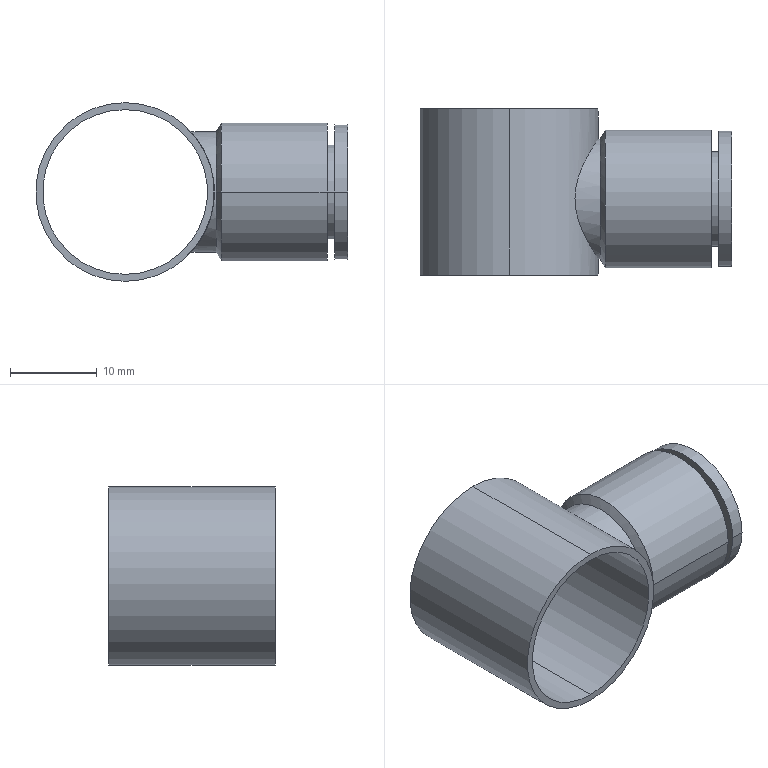Part | SolidWorks | features RefAxis 3, BaseBody 1 | 1 solid | 22 faces | box 36 x 19.2 x 20.6 mm | volume 2754 mm3 | cylinder 14 | plane 6 | cone 2 | commonest cylinder face diameters 10 x2 10.95 x2 13.9 x2 15.6 x2 15.9 x2 19 x2
STEP:
#1=CARTESIAN_POINT('',(0.,0.,-9.5));
#2=VERTEX_POINT('',#1);
#3=CARTESIAN_POINT('',(0.,0.,9.5));
#4=VERTEX_POINT('',#3);
#5=CARTESIAN_POINT('',(0.,0.,0.));
#6=DIRECTION('',(0.,1.,0.));
#7=DIRECTION('',(0.,0.,1.));
#8=AXIS2_PLACEMENT_3D('',#5,#6,#7);
#9=CIRCLE('',#8,9.5);
#10=EDGE_CURVE('',#2,#4,#9,.T.);
#11=ORIENTED_EDGE('',*,*,#10,.F.);
#12=CARTESIAN_POINT('',(0.,19.2,-9.5));
#13=VERTEX_POINT('',#12);
#14=CARTESIAN_POINT('',(0.,0.,-9.5));
#15=DIRECTION('',(0.,1.,0.));
#16=VECTOR('',#15,1000.);
#17=LINE('',#14,#16);
#18=EDGE_CURVE('',#2,#13,#17,.T.);
#19=ORIENTED_EDGE('',*,*,#18,.T.);
#20=CARTESIAN_POINT('',(0.,19.2,9.5));
#21=VERTEX_POINT('',#20);
#22=CARTESIAN_POINT('',(0.,19.2,0.));
#23=DIRECTION('',(0.,-1.,0.));
#24=DIRECTION('',(0.,0.,1.));
#25=AXIS2_PLACEMENT_3D('',#22,#23,#24);
#26=CIRCLE('',#25,9.5);
#27=EDGE_CURVE('',#21,#13,#26,.T.);
#28=ORIENTED_EDGE('',*,*,#27,.F.);
#29=CARTESIAN_POINT('',(0.,0.,9.5));
#30=DIRECTION('',(0.,1.,0.));
#31=VECTOR('',#30,1000.);
#32=LINE('',#29,#31);
#33=EDGE_CURVE('',#4,#21,#32,.T.);
#34=ORIENTED_EDGE('',*,*,#33,.F.);
#35=EDGE_LOOP('',(#11,#19,#28,#34));
#36=FACE_OUTER_BOUND('',#35,.T.);
#37=CARTESIAN_POINT('',(0.,0.,0.));
#38=DIRECTION('',(0.,1.,0.));
#39=DIRECTION('',(0.,0.,1.));
#40=AXIS2_PLACEMENT_3D('',#37,#38,#39);
#41=CYLINDRICAL_SURFACE('',#40,9.5);
#42=ADVANCED_FACE('',(#36),#41,.F.);
#43=CARTESIAN_POINT('',(10.3,1.85,0.));
#44=VERTEX_POINT('',#43);
#45=CARTESIAN_POINT('',(10.3,15.75,0.));
#46=VERTEX_POINT('',#45);
#47=CARTESIAN_POINT('',(10.3,1.85,0.));
#48=CARTESIAN_POINT('',(10.3,1.85,0.2364));
#49=CARTESIAN_POINT('',(10.292,1.862,0.4747));
#50=CARTESIAN_POINT('',(10.26,1.91,0.9419));
#51=CARTESIAN_POINT('',(10.236,1.946,1.173));
#52=CARTESIAN_POINT('',(10.142,2.086,1.856));
#53=CARTESIAN_POINT('',(10.048,2.227,2.305));
#54=CARTESIAN_POINT('',(9.818,2.585,3.145));
#55=CARTESIAN_POINT('',(9.681,2.802,3.54));
#56=CARTESIAN_POINT('',(9.376,3.308,4.283));
#57=CARTESIAN_POINT('',(9.212,3.591,4.621));
#58=CARTESIAN_POINT('',(8.874,4.213,5.24));
#59=CARTESIAN_POINT('',(8.7,4.557,5.522));
#60=CARTESIAN_POINT('',(8.368,5.287,6.013));
#61=CARTESIAN_POINT('',(8.21,5.674,6.223));
#62=CARTESIAN_POINT('',(7.933,6.5,6.574));
#63=CARTESIAN_POINT('',(7.812,6.944,6.713));
#64=CARTESIAN_POINT('',(7.689,7.624,6.854));
#65=CARTESIAN_POINT('',(7.657,7.854,6.889));
#66=CARTESIAN_POINT('',(7.613,8.322,6.938));
#67=CARTESIAN_POINT('',(7.602,8.561,6.95));
#68=CARTESIAN_POINT('',(7.602,9.269,6.95));
#69=CARTESIAN_POINT('',(7.646,9.734,6.903));
#70=CARTESIAN_POINT('',(7.811,10.651,6.715));
#71=CARTESIAN_POINT('',(7.929,11.089,6.578));
#72=CARTESIAN_POINT('',(8.138,11.713,6.314));
#73=CARTESIAN_POINT('',(8.214,11.917,6.216));
#74=CARTESIAN_POINT('',(8.371,12.309,6.003));
#75=CARTESIAN_POINT('',(8.452,12.498,5.889));
#76=CARTESIAN_POINT('',(8.7,13.044,5.521));
#77=CARTESIAN_POINT('',(8.872,13.382,5.244));
#78=CARTESIAN_POINT('',(9.127,13.852,4.777));
#79=CARTESIAN_POINT('',(9.211,14.003,4.613));
#80=CARTESIAN_POINT('',(9.374,14.285,4.273));
#81=CARTESIAN_POINT('',(9.452,14.418,4.097));
#82=CARTESIAN_POINT('',(9.678,14.793,3.548));
#83=CARTESIAN_POINT('',(9.815,15.01,3.155));
#84=CARTESIAN_POINT('',(10.048,15.372,2.307));
#85=CARTESIAN_POINT('',(10.14,15.511,1.865));
#86=CARTESIAN_POINT('',(10.266,15.7,0.9518));
#87=CARTESIAN_POINT('',(10.3,15.75,0.4749));
#88=CARTESIAN_POINT('',(10.3,15.75,0.));
#89=B_SPLINE_CURVE_WITH_KNOTS('',3,(#47,#48,#49,#50,#51,#52,#53,#54,#55,#56,#57,#58,#59,#60,#61,#62,#63,#64,#65,#66,#67,#68,#69,#70,#71,#72,#73,#74,#75,#76,#77,#78,#79,#80,#81,#82,#83,#84,#85,#86,#87,#88),.UNSPECIFIED.,.F.,.F.,(4,2,2,2,2,2,2,2,2,2,2,2,2,2,2,2,2,2,2,2,4),(0.02215,0.02285,0.02355,0.02495,0.02635,0.02775,0.02915,0.03055,0.03196,0.03266,0.03336,0.03476,0.03616,0.03686,0.03756,0.03896,0.03966,0.04036,0.04176,0.04317,0.04457),.UNSPECIFIED.);
#90=EDGE_CURVE('',#44,#46,#89,.T.);
#91=ORIENTED_EDGE('',*,*,#90,.T.);
#92=CARTESIAN_POINT('',(10.3,15.75,0.));
#93=CARTESIAN_POINT('',(10.3,15.75,-0.2383));
#94=CARTESIAN_POINT('',(10.292,15.738,-0.4775));
#95=CARTESIAN_POINT('',(10.259,15.689,-0.9459));
#96=CARTESIAN_POINT('',(10.235,15.654,-1.177));
#97=CARTESIAN_POINT('',(10.173,15.56,-1.632));
#98=CARTESIAN_POINT('',(10.134,15.502,-1.856));
#99=CARTESIAN_POINT('',(10.043,15.363,-2.298));
#100=CARTESIAN_POINT('',(9.99,15.283,-2.516));
#101=CARTESIAN_POINT('',(9.817,15.013,-3.148));
#102=CARTESIAN_POINT('',(9.68,14.796,-3.542));
#103=CARTESIAN_POINT('',(9.452,14.418,-4.097));
#104=CARTESIAN_POINT('',(9.372,14.283,-4.276));
#105=CARTESIAN_POINT('',(9.209,13.999,-4.617));
#106=CARTESIAN_POINT('',(9.126,13.851,-4.779));
#107=CARTESIAN_POINT('',(8.873,13.383,-5.243));
#108=CARTESIAN_POINT('',(8.7,13.043,-5.522));
#109=CARTESIAN_POINT('',(8.365,12.307,-6.017));
#110=CARTESIAN_POINT('',(8.208,11.919,-6.227));
#111=CARTESIAN_POINT('',(8.001,11.302,-6.488));
#112=CARTESIAN_POINT('',(7.937,11.091,-6.566));
#113=CARTESIAN_POINT('',(7.822,10.654,-6.702));
#114=CARTESIAN_POINT('',(7.771,10.428,-6.761));
#115=CARTESIAN_POINT('',(7.647,9.742,-6.902));
#116=CARTESIAN_POINT('',(7.602,9.277,-6.95));
#117=CARTESIAN_POINT('',(7.602,8.562,-6.95));
#118=CARTESIAN_POINT('',(7.613,8.325,-6.938));
#119=CARTESIAN_POINT('',(7.656,7.858,-6.89));
#120=CARTESIAN_POINT('',(7.688,7.627,-6.854));
#121=CARTESIAN_POINT('',(7.771,7.172,-6.761));
#122=CARTESIAN_POINT('',(7.822,6.945,-6.702));
#123=CARTESIAN_POINT('',(7.937,6.507,-6.565));
#124=CARTESIAN_POINT('',(8.002,6.294,-6.486));
#125=CARTESIAN_POINT('',(8.21,5.674,-6.224));
#126=CARTESIAN_POINT('',(8.37,5.283,-6.011));
#127=CARTESIAN_POINT('',(8.705,4.546,-5.514));
#128=CARTESIAN_POINT('',(8.877,4.208,-5.235));
#129=CARTESIAN_POINT('',(9.215,3.585,-4.615));
#130=CARTESIAN_POINT('',(9.382,3.298,-4.269));
#131=CARTESIAN_POINT('',(9.684,2.798,-3.532));
#132=CARTESIAN_POINT('',(9.82,2.583,-3.139));
#133=CARTESIAN_POINT('',(10.049,2.226,-2.301));
#134=CARTESIAN_POINT('',(10.143,2.085,-1.85));
#135=CARTESIAN_POINT('',(10.267,1.898,-0.939));
#136=CARTESIAN_POINT('',(10.3,1.85,-0.4743));
#137=CARTESIAN_POINT('',(10.3,1.85,0.));
#138=B_SPLINE_CURVE_WITH_KNOTS('',3,(#92,#93,#94,#95,#96,#97,#98,#99,#100,#101,#102,#103,#104,#105,#106,#107,#108,#109,#110,#111,#112,#113,#114,#115,#116,#117,#118,#119,#120,#121,#122,#123,#124,#125,#126,#127,#128,#129,#130,#131,#132,#133,#134,#135,#136,#137),.UNSPECIFIED.,.F.,.F.,(4,2,2,2,2,2,2,2,2,2,2,2,2,2,2,2,2,2,2,2,2,2,4),(0.04457,0.04527,0.04597,0.04668,0.04738,0.04878,0.04949,0.05019,0.0516,0.053,0.05371,0.05441,0.05581,0.05652,0.05722,0.05792,0.05863,0.06003,0.06144,0.06284,0.06425,0.06566,0.06706),.UNSPECIFIED.);
#139=EDGE_CURVE('',#46,#44,#138,.T.);
#140=ORIENTED_EDGE('',*,*,#139,.T.);
#141=EDGE_LOOP('',(#91,#140));
#142=FACE_BOUND('',#141,.T.);
#143=CARTESIAN_POINT('',(0.,19.2,-10.3));
#144=VERTEX_POINT('',#143);
#145=CARTESIAN_POINT('',(0.,19.2,10.3));
#146=VERTEX_POINT('',#145);
#147=CARTESIAN_POINT('',(0.,19.2,0.));
#148=DIRECTION('',(0.,-1.,0.));
#149=DIRECTION('',(0.,0.,-1.));
#150=AXIS2_PLACEMENT_3D('',#147,#148,#149);
#151=CIRCLE('',#150,10.3);
#152=EDGE_CURVE('',#144,#146,#151,.T.);
#153=ORIENTED_EDGE('',*,*,#152,.T.);
#154=CARTESIAN_POINT('',(0.,0.,10.3));
#155=VERTEX_POINT('',#154);
#156=CARTESIAN_POINT('',(0.,19.2,10.3));
#157=DIRECTION('',(0.,-1.,0.));
#158=VECTOR('',#157,1000.);
#159=LINE('',#156,#158);
#160=EDGE_CURVE('',#146,#155,#159,.T.);
#161=ORIENTED_EDGE('',*,*,#160,.T.);
#162=CARTESIAN_POINT('',(0.,0.,-10.3));
#163=VERTEX_POINT('',#162);
#164=CARTESIAN_POINT('',(0.,0.,0.));
#165=DIRECTION('',(0.,1.,0.));
#166=DIRECTION('',(0.,0.,-1.));
#167=AXIS2_PLACEMENT_3D('',#164,#165,#166);
#168=CIRCLE('',#167,10.3);
#169=EDGE_CURVE('',#155,#163,#168,.T.);
#170=ORIENTED_EDGE('',*,*,#169,.T.);
#171=CARTESIAN_POINT('',(0.,19.2,-10.3));
#172=DIRECTION('',(0.,-1.,0.));
#173=VECTOR('',#172,1000.);
#174=LINE('',#171,#173);
#175=EDGE_CURVE('',#144,#163,#174,.T.);
#176=ORIENTED_EDGE('',*,*,#175,.F.);
#177=EDGE_LOOP('',(#153,#161,#170,#176));
#178=FACE_OUTER_BOUND('',#177,.T.);
#179=CARTESIAN_POINT('',(0.,19.2,0.));
#180=DIRECTION('',(0.,-1.,0.));
#181=DIRECTION('',(0.,0.,-1.));
#182=AXIS2_PLACEMENT_3D('',#179,#180,#181);
#183=CYLINDRICAL_SURFACE('',#182,10.3);
#184=ADVANCED_FACE('',(#142,#178),#183,.T.);
#185=CARTESIAN_POINT('',(10.523,1.85,0.));
#186=VERTEX_POINT('',#185);
#187=CARTESIAN_POINT('',(10.523,15.75,0.));
#188=VERTEX_POINT('',#187);
#189=CARTESIAN_POINT('',(10.523,8.8,0.));
#190=DIRECTION('',(-1.,0.,0.));
#191=DIRECTION('',(0.,-1.,0.));
#192=AXIS2_PLACEMENT_3D('',#189,#190,#191);
#193=CIRCLE('',#192,6.95);
#194=EDGE_CURVE('',#186,#188,#193,.T.);
#195=ORIENTED_EDGE('',*,*,#194,.T.);
#196=CARTESIAN_POINT('',(25.7,15.75,0.));
#197=DIRECTION('',(-1.,0.,0.));
#198=VECTOR('',#197,1000.);
#199=LINE('',#196,#198);
#200=EDGE_CURVE('',#188,#46,#199,.T.);
#201=ORIENTED_EDGE('',*,*,#200,.T.);
#202=ORIENTED_EDGE('',*,*,#90,.F.);
#203=CARTESIAN_POINT('',(25.7,1.85,0.));
#204=DIRECTION('',(-1.,0.,0.));
#205=VECTOR('',#204,1000.);
#206=LINE('',#203,#205);
#207=EDGE_CURVE('',#186,#44,#206,.T.);
#208=ORIENTED_EDGE('',*,*,#207,.F.);
#209=EDGE_LOOP('',(#195,#201,#202,#208));
#210=FACE_OUTER_BOUND('',#209,.T.);
#211=CARTESIAN_POINT('',(25.7,8.8,0.));
#212=DIRECTION('',(-1.,0.,0.));
#213=DIRECTION('',(0.,-1.,0.));
#214=AXIS2_PLACEMENT_3D('',#211,#212,#213);
#215=CYLINDRICAL_SURFACE('',#214,6.95);
#216=ADVANCED_FACE('',(#210),#215,.T.);
#217=ORIENTED_EDGE('',*,*,#194,.F.);
#218=CARTESIAN_POINT('',(11.1,0.85,0.));
#219=VERTEX_POINT('',#218);
#220=CARTESIAN_POINT('',(11.1,0.85,0.));
#221=DIRECTION('',(0.5,-0.866,0.));
#222=VECTOR('',#221,1000.);
#223=LINE('',#220,#222);
#224=EDGE_CURVE('',#186,#219,#223,.T.);
#225=ORIENTED_EDGE('',*,*,#224,.T.);
#226=CARTESIAN_POINT('',(11.1,16.75,0.));
#227=VERTEX_POINT('',#226);
#228=CARTESIAN_POINT('',(11.1,8.8,0.));
#229=DIRECTION('',(-1.,0.,0.));
#230=DIRECTION('',(0.,1.,0.));
#231=AXIS2_PLACEMENT_3D('',#228,#229,#230);
#232=CIRCLE('',#231,7.95);
#233=EDGE_CURVE('',#219,#227,#232,.T.);
#234=ORIENTED_EDGE('',*,*,#233,.T.);
#235=CARTESIAN_POINT('',(11.1,16.75,0.));
#236=DIRECTION('',(0.5,0.866,0.));
#237=VECTOR('',#236,1000.);
#238=LINE('',#235,#237);
#239=EDGE_CURVE('',#188,#227,#238,.T.);
#240=ORIENTED_EDGE('',*,*,#239,.F.);
#241=EDGE_LOOP('',(#217,#225,#234,#240));
#242=FACE_OUTER_BOUND('',#241,.T.);
#243=CARTESIAN_POINT('',(11.1,8.8,0.));
#244=DIRECTION('',(1.,0.,0.));
#245=DIRECTION('',(0.,1.,0.));
#246=AXIS2_PLACEMENT_3D('',#243,#244,#245);
#247=CONICAL_SURFACE('',#246,7.95,1.047);
#248=ADVANCED_FACE('',(#242),#247,.T.);
#249=CARTESIAN_POINT('',(23.3,0.85,0.));
#250=VERTEX_POINT('',#249);
#251=CARTESIAN_POINT('',(23.3,16.75,0.));
#252=VERTEX_POINT('',#251);
#253=CARTESIAN_POINT('',(23.3,8.8,0.));
#254=DIRECTION('',(-1.,0.,0.));
#255=DIRECTION('',(0.,-1.,0.));
#256=AXIS2_PLACEMENT_3D('',#253,#254,#255);
#257=CIRCLE('',#256,7.95);
#258=EDGE_CURVE('',#250,#252,#257,.T.);
#259=ORIENTED_EDGE('',*,*,#258,.T.);
#260=CARTESIAN_POINT('',(25.7,16.75,0.));
#261=DIRECTION('',(-1.,0.,0.));
#262=VECTOR('',#261,1000.);
#263=LINE('',#260,#262);
#264=EDGE_CURVE('',#252,#227,#263,.T.);
#265=ORIENTED_EDGE('',*,*,#264,.T.);
#266=ORIENTED_EDGE('',*,*,#233,.F.);
#267=CARTESIAN_POINT('',(25.7,0.85,0.));
#268=DIRECTION('',(-1.,0.,0.));
#269=VECTOR('',#268,1000.);
#270=LINE('',#267,#269);
#271=EDGE_CURVE('',#250,#219,#270,.T.);
#272=ORIENTED_EDGE('',*,*,#271,.F.);
#273=EDGE_LOOP('',(#259,#265,#266,#272));
#274=FACE_OUTER_BOUND('',#273,.T.);
#275=CARTESIAN_POINT('',(25.7,8.8,0.));
#276=DIRECTION('',(-1.,0.,0.));
#277=DIRECTION('',(0.,-1.,0.));
#278=AXIS2_PLACEMENT_3D('',#275,#276,#277);
#279=CYLINDRICAL_SURFACE('',#278,7.95);
#280=ADVANCED_FACE('',(#274),#279,.T.);
#281=CARTESIAN_POINT('',(24.2,3.325,0.));
#282=VERTEX_POINT('',#281);
#283=CARTESIAN_POINT('',(24.2,14.275,0.));
#284=VERTEX_POINT('',#283);
#285=CARTESIAN_POINT('',(24.2,8.8,0.));
#286=DIRECTION('',(-1.,0.,0.));
#287=DIRECTION('',(0.,-1.,0.));
#288=AXIS2_PLACEMENT_3D('',#285,#286,#287);
#289=CIRCLE('',#288,5.475);
#290=EDGE_CURVE('',#282,#284,#289,.T.);
#291=ORIENTED_EDGE('',*,*,#290,.T.);
#292=CARTESIAN_POINT('',(23.3,14.275,0.));
#293=VERTEX_POINT('',#292);
#294=CARTESIAN_POINT('',(25.7,14.275,0.));
#295=DIRECTION('',(-1.,0.,0.));
#296=VECTOR('',#295,1000.);
#297=LINE('',#294,#296);
#298=EDGE_CURVE('',#284,#293,#297,.T.);
#299=ORIENTED_EDGE('',*,*,#298,.T.);
#300=CARTESIAN_POINT('',(23.3,3.325,0.));
#301=VERTEX_POINT('',#300);
#302=CARTESIAN_POINT('',(23.3,8.8,0.));
#303=DIRECTION('',(1.,0.,0.));
#304=DIRECTION('',(0.,-1.,0.));
#305=AXIS2_PLACEMENT_3D('',#302,#303,#304);
#306=CIRCLE('',#305,5.475);
#307=EDGE_CURVE('',#293,#301,#306,.T.);
#308=ORIENTED_EDGE('',*,*,#307,.T.);
#309=CARTESIAN_POINT('',(25.7,3.325,0.));
#310=DIRECTION('',(-1.,0.,0.));
#311=VECTOR('',#310,1000.);
#312=LINE('',#309,#311);
#313=EDGE_CURVE('',#282,#301,#312,.T.);
#314=ORIENTED_EDGE('',*,*,#313,.F.);
#315=EDGE_LOOP('',(#291,#299,#308,#314));
#316=FACE_OUTER_BOUND('',#315,.T.);
#317=CARTESIAN_POINT('',(25.7,8.8,0.));
#318=DIRECTION('',(-1.,0.,0.));
#319=DIRECTION('',(0.,-1.,0.));
#320=AXIS2_PLACEMENT_3D('',#317,#318,#319);
#321=CYLINDRICAL_SURFACE('',#320,5.475);
#322=ADVANCED_FACE('',(#316),#321,.T.);
#323=CARTESIAN_POINT('',(25.7,1.,0.));
#324=VERTEX_POINT('',#323);
#325=CARTESIAN_POINT('',(25.7,16.6,0.));
#326=VERTEX_POINT('',#325);
#327=CARTESIAN_POINT('',(25.7,8.8,0.));
#328=DIRECTION('',(-1.,0.,0.));
#329=DIRECTION('',(0.,-1.,0.));
#330=AXIS2_PLACEMENT_3D('',#327,#328,#329);
#331=CIRCLE('',#330,7.8);
#332=EDGE_CURVE('',#324,#326,#331,.T.);
#333=ORIENTED_EDGE('',*,*,#332,.T.);
#334=CARTESIAN_POINT('',(24.2,16.6,0.));
#335=VERTEX_POINT('',#334);
#336=CARTESIAN_POINT('',(25.7,16.6,0.));
#337=DIRECTION('',(-1.,0.,0.));
#338=VECTOR('',#337,1000.);
#339=LINE('',#336,#338);
#340=EDGE_CURVE('',#326,#335,#339,.T.);
#341=ORIENTED_EDGE('',*,*,#340,.T.);
#342=CARTESIAN_POINT('',(24.2,1.,0.));
#343=VERTEX_POINT('',#342);
#344=CARTESIAN_POINT('',(24.2,8.8,0.));
#345=DIRECTION('',(1.,0.,0.));
#346=DIRECTION('',(0.,-1.,0.));
#347=AXIS2_PLACEMENT_3D('',#344,#345,#346);
#348=CIRCLE('',#347,7.8);
#349=EDGE_CURVE('',#335,#343,#348,.T.);
#350=ORIENTED_EDGE('',*,*,#349,.T.);
#351=CARTESIAN_POINT('',(25.7,1.,0.));
#352=DIRECTION('',(-1.,0.,0.));
#353=VECTOR('',#352,1000.);
#354=LINE('',#351,#353);
#355=EDGE_CURVE('',#324,#343,#354,.T.);
#356=ORIENTED_EDGE('',*,*,#355,.F.);
#357=EDGE_LOOP('',(#333,#341,#350,#356));
#358=FACE_OUTER_BOUND('',#357,.T.);
#359=CARTESIAN_POINT('',(25.7,8.8,0.));
#360=DIRECTION('',(-1.,0.,0.));
#361=DIRECTION('',(0.,-1.,0.));
#362=AXIS2_PLACEMENT_3D('',#359,#360,#361);
#363=CYLINDRICAL_SURFACE('',#362,7.8);
#364=ADVANCED_FACE('',(#358),#363,.T.);
#365=CARTESIAN_POINT('',(25.7,8.8,5.));
#366=VERTEX_POINT('',#365);
#367=CARTESIAN_POINT('',(25.7,8.8,-5.));
#368=VERTEX_POINT('',#367);
#369=CARTESIAN_POINT('',(25.7,8.8,0.));
#370=DIRECTION('',(1.,0.,0.));
#371=DIRECTION('',(0.,0.,1.));
#372=AXIS2_PLACEMENT_3D('',#369,#370,#371);
#373=CIRCLE('',#372,5.);
#374=EDGE_CURVE('',#366,#368,#373,.T.);
#375=ORIENTED_EDGE('',*,*,#374,.T.);
#376=CARTESIAN_POINT('',(10.1,8.8,-5.));
#377=VERTEX_POINT('',#376);
#378=CARTESIAN_POINT('',(10.1,8.8,-5.));
#379=DIRECTION('',(-1.,0.,0.));
#380=VECTOR('',#379,1000.);
#381=LINE('',#378,#380);
#382=EDGE_CURVE('',#368,#377,#381,.T.);
#383=ORIENTED_EDGE('',*,*,#382,.T.);
#384=CARTESIAN_POINT('',(10.1,8.8,5.));
#385=VERTEX_POINT('',#384);
#386=CARTESIAN_POINT('',(10.1,8.8,0.));
#387=DIRECTION('',(1.,0.,0.));
#388=DIRECTION('',(0.,0.,1.));
#389=AXIS2_PLACEMENT_3D('',#386,#387,#388);
#390=CIRCLE('',#389,5.);
#391=EDGE_CURVE('',#385,#377,#390,.T.);
#392=ORIENTED_EDGE('',*,*,#391,.F.);
#393=CARTESIAN_POINT('',(10.1,8.8,5.));
#394=DIRECTION('',(-1.,0.,0.));
#395=VECTOR('',#394,1000.);
#396=LINE('',#393,#395);
#397=EDGE_CURVE('',#366,#385,#396,.T.);
#398=ORIENTED_EDGE('',*,*,#397,.F.);
#399=EDGE_LOOP('',(#375,#383,#392,#398));
#400=FACE_OUTER_BOUND('',#399,.T.);
#401=CARTESIAN_POINT('',(10.1,8.8,0.));
#402=DIRECTION('',(-1.,0.,0.));
#403=DIRECTION('',(0.,0.,1.));
#404=AXIS2_PLACEMENT_3D('',#401,#402,#403);
#405=CYLINDRICAL_SURFACE('',#404,5.);
#406=ADVANCED_FACE('',(#400),#405,.F.);
#407=ORIENTED_EDGE('',*,*,#18,.F.);
#408=CARTESIAN_POINT('',(0.,0.,0.));
#409=DIRECTION('',(0.,1.,0.));
#410=DIRECTION('',(0.,0.,1.));
#411=AXIS2_PLACEMENT_3D('',#408,#409,#410);
#412=CIRCLE('',#411,9.5);
#413=EDGE_CURVE('',#4,#2,#412,.T.);
#414=ORIENTED_EDGE('',*,*,#413,.F.);
#415=ORIENTED_EDGE('',*,*,#33,.T.);
#416=CARTESIAN_POINT('',(0.,19.2,0.));
#417=DIRECTION('',(0.,-1.,0.));
#418=DIRECTION('',(0.,0.,1.));
#419=AXIS2_PLACEMENT_3D('',#416,#417,#418);
#420=CIRCLE('',#419,9.5);
#421=EDGE_CURVE('',#13,#21,#420,.T.);
#422=ORIENTED_EDGE('',*,*,#421,.F.);
#423=EDGE_LOOP('',(#407,#414,#415,#422));
#424=FACE_OUTER_BOUND('',#423,.T.);
#425=CARTESIAN_POINT('',(0.,0.,0.));
#426=DIRECTION('',(0.,1.,0.));
#427=DIRECTION('',(0.,0.,1.));
#428=AXIS2_PLACEMENT_3D('',#425,#426,#427);
#429=CYLINDRICAL_SURFACE('',#428,9.5);
#430=ADVANCED_FACE('',(#424),#429,.F.);
#431=ORIENTED_EDGE('',*,*,#152,.F.);
#432=CARTESIAN_POINT('',(0.,19.2,0.));
#433=DIRECTION('',(0.,-1.,0.));
#434=DIRECTION('',(0.,0.,-1.));
#435=AXIS2_PLACEMENT_3D('',#432,#433,#434);
#436=CIRCLE('',#435,10.3);
#437=EDGE_CURVE('',#146,#144,#436,.T.);
#438=ORIENTED_EDGE('',*,*,#437,.F.);
#439=EDGE_LOOP('',(#431,#438));
#440=FACE_OUTER_BOUND('',#439,.T.);
#441=ORIENTED_EDGE('',*,*,#27,.T.);
#442=ORIENTED_EDGE('',*,*,#421,.T.);
#443=EDGE_LOOP('',(#441,#442));
#444=FACE_BOUND('',#443,.T.);
#445=CARTESIAN_POINT('',(-10.3,19.2,0.));
#446=DIRECTION('',(0.,-1.,0.));
#447=DIRECTION('',(0.,0.,-1.));
#448=AXIS2_PLACEMENT_3D('',#445,#446,#447);
#449=PLANE('',#448);
#450=ADVANCED_FACE('',(#440,#444),#449,.F.);
#451=ORIENTED_EDGE('',*,*,#413,.T.);
#452=ORIENTED_EDGE('',*,*,#10,.T.);
#453=EDGE_LOOP('',(#451,#452));
#454=FACE_BOUND('',#453,.T.);
#455=CARTESIAN_POINT('',(0.,0.,0.));
#456=DIRECTION('',(0.,1.,0.));
#457=DIRECTION('',(0.,0.,-1.));
#458=AXIS2_PLACEMENT_3D('',#455,#456,#457);
#459=CIRCLE('',#458,10.3);
#460=EDGE_CURVE('',#163,#155,#459,.T.);
#461=ORIENTED_EDGE('',*,*,#460,.F.);
#462=ORIENTED_EDGE('',*,*,#169,.F.);
#463=EDGE_LOOP('',(#461,#462));
#464=FACE_OUTER_BOUND('',#463,.T.);
#465=CARTESIAN_POINT('',(0.,0.,0.));
#466=DIRECTION('',(0.,1.,0.));
#467=DIRECTION('',(0.,0.,1.));
#468=AXIS2_PLACEMENT_3D('',#465,#466,#467);
#469=PLANE('',#468);
#470=ADVANCED_FACE('',(#454,#464),#469,.F.);
#471=ORIENTED_EDGE('',*,*,#160,.F.);
#472=ORIENTED_EDGE('',*,*,#437,.T.);
#473=ORIENTED_EDGE('',*,*,#175,.T.);
#474=ORIENTED_EDGE('',*,*,#460,.T.);
#475=EDGE_LOOP('',(#471,#472,#473,#474));
#476=FACE_OUTER_BOUND('',#475,.T.);
#477=CARTESIAN_POINT('',(0.,19.2,0.));
#478=DIRECTION('',(0.,-1.,0.));
#479=DIRECTION('',(0.,0.,-1.));
#480=AXIS2_PLACEMENT_3D('',#477,#478,#479);
#481=CYLINDRICAL_SURFACE('',#480,10.3);
#482=ADVANCED_FACE('',(#476),#481,.T.);
#483=ORIENTED_EDGE('',*,*,#200,.F.);
#484=CARTESIAN_POINT('',(10.523,8.8,0.));
#485=DIRECTION('',(-1.,0.,0.));
#486=DIRECTION('',(0.,-1.,0.));
#487=AXIS2_PLACEMENT_3D('',#484,#485,#486);
#488=CIRCLE('',#487,6.95);
#489=EDGE_CURVE('',#188,#186,#488,.T.);
#490=ORIENTED_EDGE('',*,*,#489,.T.);
#491=ORIENTED_EDGE('',*,*,#207,.T.);
#492=ORIENTED_EDGE('',*,*,#139,.F.);
#493=EDGE_LOOP('',(#483,#490,#491,#492));
#494=FACE_OUTER_BOUND('',#493,.T.);
#495=CARTESIAN_POINT('',(25.7,8.8,0.));
#496=DIRECTION('',(-1.,0.,0.));
#497=DIRECTION('',(0.,-1.,0.));
#498=AXIS2_PLACEMENT_3D('',#495,#496,#497);
#499=CYLINDRICAL_SURFACE('',#498,6.95);
#500=ADVANCED_FACE('',(#494),#499,.T.);
#501=ORIENTED_EDGE('',*,*,#224,.F.);
#502=ORIENTED_EDGE('',*,*,#489,.F.);
#503=ORIENTED_EDGE('',*,*,#239,.T.);
#504=CARTESIAN_POINT('',(11.1,8.8,0.));
#505=DIRECTION('',(-1.,0.,0.));
#506=DIRECTION('',(0.,1.,0.));
#507=AXIS2_PLACEMENT_3D('',#504,#505,#506);
#508=CIRCLE('',#507,7.95);
#509=EDGE_CURVE('',#227,#219,#508,.T.);
#510=ORIENTED_EDGE('',*,*,#509,.T.);
#511=EDGE_LOOP('',(#501,#502,#503,#510));
#512=FACE_OUTER_BOUND('',#511,.T.);
#513=CARTESIAN_POINT('',(11.1,8.8,0.));
#514=DIRECTION('',(1.,0.,0.));
#515=DIRECTION('',(0.,1.,0.));
#516=AXIS2_PLACEMENT_3D('',#513,#514,#515);
#517=CONICAL_SURFACE('',#516,7.95,1.047);
#518=ADVANCED_FACE('',(#512),#517,.T.);
#519=ORIENTED_EDGE('',*,*,#264,.F.);
#520=CARTESIAN_POINT('',(23.3,8.8,0.));
#521=DIRECTION('',(-1.,0.,0.));
#522=DIRECTION('',(0.,-1.,0.));
#523=AXIS2_PLACEMENT_3D('',#520,#521,#522);
#524=CIRCLE('',#523,7.95);
#525=EDGE_CURVE('',#252,#250,#524,.T.);
#526=ORIENTED_EDGE('',*,*,#525,.T.);
#527=ORIENTED_EDGE('',*,*,#271,.T.);
#528=ORIENTED_EDGE('',*,*,#509,.F.);
#529=EDGE_LOOP('',(#519,#526,#527,#528));
#530=FACE_OUTER_BOUND('',#529,.T.);
#531=CARTESIAN_POINT('',(25.7,8.8,0.));
#532=DIRECTION('',(-1.,0.,0.));
#533=DIRECTION('',(0.,-1.,0.));
#534=AXIS2_PLACEMENT_3D('',#531,#532,#533);
#535=CYLINDRICAL_SURFACE('',#534,7.95);
#536=ADVANCED_FACE('',(#530),#535,.T.);
#537=ORIENTED_EDGE('',*,*,#258,.F.);
#538=ORIENTED_EDGE('',*,*,#525,.F.);
#539=EDGE_LOOP('',(#537,#538));
#540=FACE_OUTER_BOUND('',#539,.T.);
#541=CARTESIAN_POINT('',(23.3,8.8,0.));
#542=DIRECTION('',(1.,0.,0.));
#543=DIRECTION('',(0.,-1.,0.));
#544=AXIS2_PLACEMENT_3D('',#541,#542,#543);
#545=CIRCLE('',#544,5.475);
#546=EDGE_CURVE('',#301,#293,#545,.T.);
#547=ORIENTED_EDGE('',*,*,#546,.F.);
#548=ORIENTED_EDGE('',*,*,#307,.F.);
#549=EDGE_LOOP('',(#547,#548));
#550=FACE_BOUND('',#549,.T.);
#551=CARTESIAN_POINT('',(23.3,16.75,0.));
#552=DIRECTION('',(-1.,0.,0.));
#553=DIRECTION('',(0.,-1.,0.));
#554=AXIS2_PLACEMENT_3D('',#551,#552,#553);
#555=PLANE('',#554);
#556=ADVANCED_FACE('',(#540,#550),#555,.F.);
#557=ORIENTED_EDGE('',*,*,#298,.F.);
#558=CARTESIAN_POINT('',(24.2,8.8,0.));
#559=DIRECTION('',(-1.,0.,0.));
#560=DIRECTION('',(0.,-1.,0.));
#561=AXIS2_PLACEMENT_3D('',#558,#559,#560);
#562=CIRCLE('',#561,5.475);
#563=EDGE_CURVE('',#284,#282,#562,.T.);
#564=ORIENTED_EDGE('',*,*,#563,.T.);
#565=ORIENTED_EDGE('',*,*,#313,.T.);
#566=ORIENTED_EDGE('',*,*,#546,.T.);
#567=EDGE_LOOP('',(#557,#564,#565,#566));
#568=FACE_OUTER_BOUND('',#567,.T.);
#569=CARTESIAN_POINT('',(25.7,8.8,0.));
#570=DIRECTION('',(-1.,0.,0.));
#571=DIRECTION('',(0.,-1.,0.));
#572=AXIS2_PLACEMENT_3D('',#569,#570,#571);
#573=CYLINDRICAL_SURFACE('',#572,5.475);
#574=ADVANCED_FACE('',(#568),#573,.T.);
#575=ORIENTED_EDGE('',*,*,#290,.F.);
#576=ORIENTED_EDGE('',*,*,#563,.F.);
#577=EDGE_LOOP('',(#575,#576));
#578=FACE_BOUND('',#577,.T.);
#579=CARTESIAN_POINT('',(24.2,8.8,0.));
#580=DIRECTION('',(1.,0.,0.));
#581=DIRECTION('',(0.,-1.,0.));
#582=AXIS2_PLACEMENT_3D('',#579,#580,#581);
#583=CIRCLE('',#582,7.8);
#584=EDGE_CURVE('',#343,#335,#583,.T.);
#585=ORIENTED_EDGE('',*,*,#584,.F.);
#586=ORIENTED_EDGE('',*,*,#349,.F.);
#587=EDGE_LOOP('',(#585,#586));
#588=FACE_OUTER_BOUND('',#587,.T.);
#589=CARTESIAN_POINT('',(24.2,14.275,0.));
#590=DIRECTION('',(1.,0.,0.));
#591=DIRECTION('',(0.,1.,0.));
#592=AXIS2_PLACEMENT_3D('',#589,#590,#591);
#593=PLANE('',#592);
#594=ADVANCED_FACE('',(#578,#588),#593,.F.);
#595=ORIENTED_EDGE('',*,*,#340,.F.);
#596=CARTESIAN_POINT('',(25.7,8.8,0.));
#597=DIRECTION('',(-1.,0.,0.));
#598=DIRECTION('',(0.,-1.,0.));
#599=AXIS2_PLACEMENT_3D('',#596,#597,#598);
#600=CIRCLE('',#599,7.8);
#601=EDGE_CURVE('',#326,#324,#600,.T.);
#602=ORIENTED_EDGE('',*,*,#601,.T.);
#603=ORIENTED_EDGE('',*,*,#355,.T.);
#604=ORIENTED_EDGE('',*,*,#584,.T.);
#605=EDGE_LOOP('',(#595,#602,#603,#604));
#606=FACE_OUTER_BOUND('',#605,.T.);
#607=CARTESIAN_POINT('',(25.7,8.8,0.));
#608=DIRECTION('',(-1.,0.,0.));
#609=DIRECTION('',(0.,-1.,0.));
#610=AXIS2_PLACEMENT_3D('',#607,#608,#609);
#611=CYLINDRICAL_SURFACE('',#610,7.8);
#612=ADVANCED_FACE('',(#606),#611,.T.);
#613=ORIENTED_EDGE('',*,*,#332,.F.);
#614=ORIENTED_EDGE('',*,*,#601,.F.);
#615=EDGE_LOOP('',(#613,#614));
#616=FACE_OUTER_BOUND('',#615,.T.);
#617=ORIENTED_EDGE('',*,*,#374,.F.);
#618=CARTESIAN_POINT('',(25.7,8.8,0.));
#619=DIRECTION('',(1.,0.,0.));
#620=DIRECTION('',(0.,0.,1.));
#621=AXIS2_PLACEMENT_3D('',#618,#619,#620);
#622=CIRCLE('',#621,5.);
#623=EDGE_CURVE('',#368,#366,#622,.T.);
#624=ORIENTED_EDGE('',*,*,#623,.F.);
#625=EDGE_LOOP('',(#617,#624));
#626=FACE_BOUND('',#625,.T.);
#627=CARTESIAN_POINT('',(25.7,16.6,0.));
#628=DIRECTION('',(-1.,0.,0.));
#629=DIRECTION('',(0.,-1.,0.));
#630=AXIS2_PLACEMENT_3D('',#627,#628,#629);
#631=PLANE('',#630);
#632=ADVANCED_FACE('',(#616,#626),#631,.F.);
#633=ORIENTED_EDGE('',*,*,#382,.F.);
#634=ORIENTED_EDGE('',*,*,#623,.T.);
#635=ORIENTED_EDGE('',*,*,#397,.T.);
#636=CARTESIAN_POINT('',(10.1,8.8,0.));
#637=DIRECTION('',(1.,0.,0.));
#638=DIRECTION('',(0.,0.,1.));
#639=AXIS2_PLACEMENT_3D('',#636,#637,#638);
#640=CIRCLE('',#639,5.);
#641=EDGE_CURVE('',#377,#385,#640,.T.);
#642=ORIENTED_EDGE('',*,*,#641,.F.);
#643=EDGE_LOOP('',(#633,#634,#635,#642));
#644=FACE_OUTER_BOUND('',#643,.T.);
#645=CARTESIAN_POINT('',(10.1,8.8,0.));
#646=DIRECTION('',(-1.,0.,0.));
#647=DIRECTION('',(0.,0.,1.));
#648=AXIS2_PLACEMENT_3D('',#645,#646,#647);
#649=CYLINDRICAL_SURFACE('',#648,5.);
#650=ADVANCED_FACE('',(#644),#649,.F.);
#651=ORIENTED_EDGE('',*,*,#391,.T.);
#652=ORIENTED_EDGE('',*,*,#641,.T.);
#653=EDGE_LOOP('',(#651,#652));
#654=FACE_OUTER_BOUND('',#653,.T.);
#655=CARTESIAN_POINT('',(10.1,8.8,0.));
#656=DIRECTION('',(1.,0.,0.));
#657=DIRECTION('',(0.,0.,-1.));
#658=AXIS2_PLACEMENT_3D('',#655,#656,#657);
#659=PLANE('',#658);
#660=ADVANCED_FACE('',(#654),#659,.T.);
#661=CLOSED_SHELL('',(#42,#184,#216,#248,#280,#322,#364,#406,#430,#450,#470,#482,#500,#518,#536,#556,#574,#594,#612,#632,#650,#660));
#662=MANIFOLD_SOLID_BREP('',#661);
#663=CARTESIAN_POINT('',(0.,0.,0.));
#664=DIRECTION('',(0.,0.,1.));
#665=DIRECTION('',(1.,0.,0.));
#666=AXIS2_PLACEMENT_3D('',#663,#664,#665);
#667=(LENGTH_UNIT()NAMED_UNIT(*)SI_UNIT(.MILLI.,.METRE.));
#668=UNCERTAINTY_MEASURE_WITH_UNIT(LENGTH_MEASURE(0.00001),#667,'','');
#669=(NAMED_UNIT(*)PLANE_ANGLE_UNIT()SI_UNIT($,.RADIAN.));
#670=(NAMED_UNIT(*)SI_UNIT($,.STERADIAN.)SOLID_ANGLE_UNIT());
#671=(GEOMETRIC_REPRESENTATION_CONTEXT(3)GLOBAL_UNCERTAINTY_ASSIGNED_CONTEXT((#668))GLOBAL_UNIT_ASSIGNED_CONTEXT((#667,#669,#670))REPRESENTATION_CONTEXT('',''));
#672=ADVANCED_BREP_SHAPE_REPRESENTATION('',(#662,#666),#671);